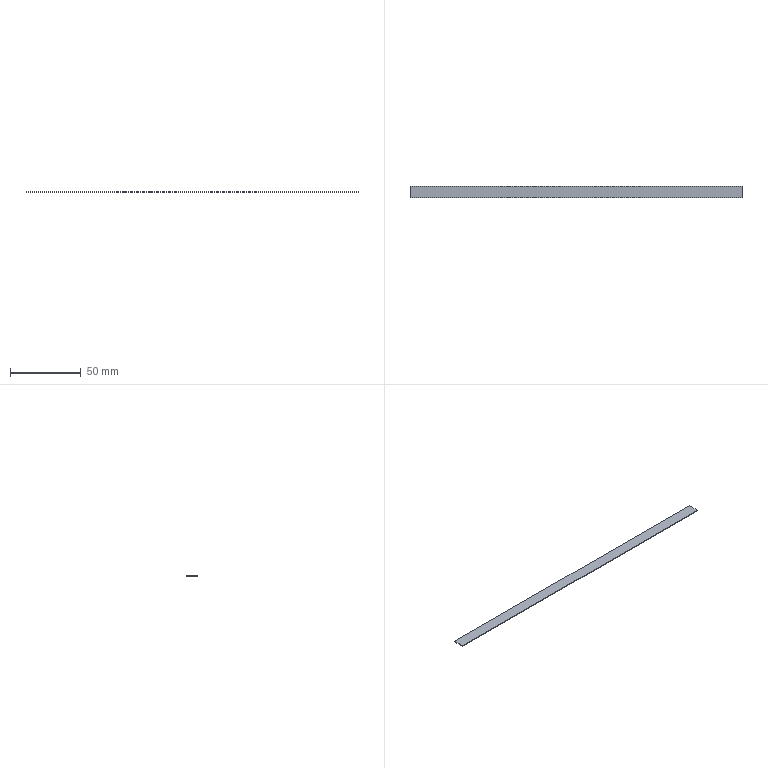Part | STEP file | 1 solid | 6 faces | box 235 x 8 x 0.5 mm | volume 940 mm3 | plane 6
STEP:
#1=CARTESIAN_POINT('',(0.,0.,0.));
#2=DIRECTION('',(0.,0.,1.));
#3=DIRECTION('',(1.,0.,0.));
#4=AXIS2_PLACEMENT_3D('',#1,#2,#3);
#5=CARTESIAN_POINT('',(117.5,-4.,0.));
#6=VERTEX_POINT('',#5);
#7=CARTESIAN_POINT('',(117.5,4.,0.));
#8=VERTEX_POINT('',#7);
#9=CARTESIAN_POINT('',(117.5,-4.,0.));
#10=DIRECTION('',(0.,1.,0.));
#11=VECTOR('',#10,1.);
#12=LINE('',#9,#11);
#13=CARTESIAN_POINT('',(0.,0.,0.));
#14=DIRECTION('',(0.,0.,-1.));
#15=DIRECTION('',(-1.,0.,0.));
#16=AXIS2_PLACEMENT_3D('',#13,#14,#15);
#17=PLANE('',#16);
#18=CARTESIAN_POINT('',(-117.5,-4.));
#19=DIRECTION('',(0.,1.));
#20=VECTOR('',#19,1.);
#21=LINE('',#18,#20);
#22=(GEOMETRIC_REPRESENTATION_CONTEXT(2)PARAMETRIC_REPRESENTATION_CONTEXT()REPRESENTATION_CONTEXT('',''));
#23=DEFINITIONAL_REPRESENTATION('',(#21),#22);
#24=PCURVE('',#17,#23);
#25=CARTESIAN_POINT('',(117.5,-4.,0.5));
#26=DIRECTION('',(-1.,0.,0.));
#27=DIRECTION('',(0.,0.,1.));
#28=AXIS2_PLACEMENT_3D('',#25,#26,#27);
#29=PLANE('',#28);
#30=CARTESIAN_POINT('',(-0.5,0.));
#31=DIRECTION('',(0.,1.));
#32=VECTOR('',#31,1.);
#33=LINE('',#30,#32);
#34=(GEOMETRIC_REPRESENTATION_CONTEXT(2)PARAMETRIC_REPRESENTATION_CONTEXT()REPRESENTATION_CONTEXT('',''));
#35=DEFINITIONAL_REPRESENTATION('',(#33),#34);
#36=PCURVE('',#29,#35);
#37=SURFACE_CURVE('',#12,(#24,#36),.PCURVE_S1.);
#38=EDGE_CURVE('',#6,#8,#37,.T.);
#39=ORIENTED_EDGE('',*,*,#38,.F.);
#40=CARTESIAN_POINT('',(-117.5,-4.,0.));
#41=VERTEX_POINT('',#40);
#42=CARTESIAN_POINT('',(-117.5,-4.,0.));
#43=DIRECTION('',(1.,0.,0.));
#44=VECTOR('',#43,1.);
#45=LINE('',#42,#44);
#46=CARTESIAN_POINT('',(117.5,-4.));
#47=DIRECTION('',(-1.,0.));
#48=VECTOR('',#47,1.);
#49=LINE('',#46,#48);
#50=(GEOMETRIC_REPRESENTATION_CONTEXT(2)PARAMETRIC_REPRESENTATION_CONTEXT()REPRESENTATION_CONTEXT('',''));
#51=DEFINITIONAL_REPRESENTATION('',(#49),#50);
#52=PCURVE('',#17,#51);
#53=CARTESIAN_POINT('',(-117.5,-4.,0.5));
#54=DIRECTION('',(0.,1.,0.));
#55=DIRECTION('',(0.,0.,1.));
#56=AXIS2_PLACEMENT_3D('',#53,#54,#55);
#57=PLANE('',#56);
#58=CARTESIAN_POINT('',(-0.5,0.));
#59=DIRECTION('',(0.,1.));
#60=VECTOR('',#59,1.);
#61=LINE('',#58,#60);
#62=(GEOMETRIC_REPRESENTATION_CONTEXT(2)PARAMETRIC_REPRESENTATION_CONTEXT()REPRESENTATION_CONTEXT('',''));
#63=DEFINITIONAL_REPRESENTATION('',(#61),#62);
#64=PCURVE('',#57,#63);
#65=SURFACE_CURVE('',#45,(#52,#64),.PCURVE_S1.);
#66=EDGE_CURVE('',#41,#6,#65,.T.);
#67=ORIENTED_EDGE('',*,*,#66,.F.);
#68=CARTESIAN_POINT('',(-117.5,4.,0.));
#69=VERTEX_POINT('',#68);
#70=CARTESIAN_POINT('',(-117.5,-4.,0.));
#71=DIRECTION('',(0.,-1.,0.));
#72=VECTOR('',#71,1.);
#73=LINE('',#70,#72);
#74=CARTESIAN_POINT('',(117.5,-4.));
#75=DIRECTION('',(0.,-1.));
#76=VECTOR('',#75,1.);
#77=LINE('',#74,#76);
#78=(GEOMETRIC_REPRESENTATION_CONTEXT(2)PARAMETRIC_REPRESENTATION_CONTEXT()REPRESENTATION_CONTEXT('',''));
#79=DEFINITIONAL_REPRESENTATION('',(#77),#78);
#80=PCURVE('',#17,#79);
#81=CARTESIAN_POINT('',(-117.5,-4.,0.5));
#82=DIRECTION('',(1.,0.,0.));
#83=DIRECTION('',(0.,0.,-1.));
#84=AXIS2_PLACEMENT_3D('',#81,#82,#83);
#85=PLANE('',#84);
#86=CARTESIAN_POINT('',(0.5,0.));
#87=DIRECTION('',(0.,-1.));
#88=VECTOR('',#87,1.);
#89=LINE('',#86,#88);
#90=(GEOMETRIC_REPRESENTATION_CONTEXT(2)PARAMETRIC_REPRESENTATION_CONTEXT()REPRESENTATION_CONTEXT('',''));
#91=DEFINITIONAL_REPRESENTATION('',(#89),#90);
#92=PCURVE('',#85,#91);
#93=SURFACE_CURVE('',#73,(#80,#92),.PCURVE_S1.);
#94=EDGE_CURVE('',#69,#41,#93,.T.);
#95=ORIENTED_EDGE('',*,*,#94,.F.);
#96=CARTESIAN_POINT('',(-117.5,4.,0.));
#97=DIRECTION('',(-1.,0.,0.));
#98=VECTOR('',#97,1.);
#99=LINE('',#96,#98);
#100=CARTESIAN_POINT('',(117.5,4.));
#101=DIRECTION('',(1.,0.));
#102=VECTOR('',#101,1.);
#103=LINE('',#100,#102);
#104=(GEOMETRIC_REPRESENTATION_CONTEXT(2)PARAMETRIC_REPRESENTATION_CONTEXT()REPRESENTATION_CONTEXT('',''));
#105=DEFINITIONAL_REPRESENTATION('',(#103),#104);
#106=PCURVE('',#17,#105);
#107=CARTESIAN_POINT('',(-117.5,4.,0.5));
#108=DIRECTION('',(0.,-1.,0.));
#109=DIRECTION('',(0.,0.,-1.));
#110=AXIS2_PLACEMENT_3D('',#107,#108,#109);
#111=PLANE('',#110);
#112=CARTESIAN_POINT('',(0.5,0.));
#113=DIRECTION('',(0.,-1.));
#114=VECTOR('',#113,1.);
#115=LINE('',#112,#114);
#116=(GEOMETRIC_REPRESENTATION_CONTEXT(2)PARAMETRIC_REPRESENTATION_CONTEXT()REPRESENTATION_CONTEXT('',''));
#117=DEFINITIONAL_REPRESENTATION('',(#115),#116);
#118=PCURVE('',#111,#117);
#119=SURFACE_CURVE('',#99,(#106,#118),.PCURVE_S1.);
#120=EDGE_CURVE('',#8,#69,#119,.T.);
#121=ORIENTED_EDGE('',*,*,#120,.F.);
#122=EDGE_LOOP('',(#39,#67,#95,#121));
#123=FACE_BOUND('',#122,.T.);
#124=ADVANCED_FACE('',(#123),#17,.T.);
#125=CARTESIAN_POINT('',(117.5,-4.,0.5));
#126=VERTEX_POINT('',#125);
#127=CARTESIAN_POINT('',(117.5,4.,0.5));
#128=VERTEX_POINT('',#127);
#129=CARTESIAN_POINT('',(117.5,-4.,0.5));
#130=DIRECTION('',(0.,1.,0.));
#131=VECTOR('',#130,1.);
#132=LINE('',#129,#131);
#133=CARTESIAN_POINT('',(0.,0.,0.5));
#134=DIRECTION('',(0.,0.,-1.));
#135=DIRECTION('',(-1.,0.,0.));
#136=AXIS2_PLACEMENT_3D('',#133,#134,#135);
#137=PLANE('',#136);
#138=CARTESIAN_POINT('',(-117.5,-4.));
#139=DIRECTION('',(0.,1.));
#140=VECTOR('',#139,1.);
#141=LINE('',#138,#140);
#142=(GEOMETRIC_REPRESENTATION_CONTEXT(2)PARAMETRIC_REPRESENTATION_CONTEXT()REPRESENTATION_CONTEXT('',''));
#143=DEFINITIONAL_REPRESENTATION('',(#141),#142);
#144=PCURVE('',#137,#143);
#145=CARTESIAN_POINT('',(0.,0.));
#146=DIRECTION('',(0.,1.));
#147=VECTOR('',#146,1.);
#148=LINE('',#145,#147);
#149=(GEOMETRIC_REPRESENTATION_CONTEXT(2)PARAMETRIC_REPRESENTATION_CONTEXT()REPRESENTATION_CONTEXT('',''));
#150=DEFINITIONAL_REPRESENTATION('',(#148),#149);
#151=PCURVE('',#29,#150);
#152=SURFACE_CURVE('',#132,(#144,#151),.PCURVE_S1.);
#153=EDGE_CURVE('',#126,#128,#152,.T.);
#154=ORIENTED_EDGE('',*,*,#153,.T.);
#155=CARTESIAN_POINT('',(-117.5,4.,0.5));
#156=VERTEX_POINT('',#155);
#157=CARTESIAN_POINT('',(-117.5,4.,0.5));
#158=DIRECTION('',(-1.,0.,0.));
#159=VECTOR('',#158,1.);
#160=LINE('',#157,#159);
#161=CARTESIAN_POINT('',(117.5,4.));
#162=DIRECTION('',(1.,0.));
#163=VECTOR('',#162,1.);
#164=LINE('',#161,#163);
#165=(GEOMETRIC_REPRESENTATION_CONTEXT(2)PARAMETRIC_REPRESENTATION_CONTEXT()REPRESENTATION_CONTEXT('',''));
#166=DEFINITIONAL_REPRESENTATION('',(#164),#165);
#167=PCURVE('',#137,#166);
#168=CARTESIAN_POINT('',(0.,0.));
#169=DIRECTION('',(0.,-1.));
#170=VECTOR('',#169,1.);
#171=LINE('',#168,#170);
#172=(GEOMETRIC_REPRESENTATION_CONTEXT(2)PARAMETRIC_REPRESENTATION_CONTEXT()REPRESENTATION_CONTEXT('',''));
#173=DEFINITIONAL_REPRESENTATION('',(#171),#172);
#174=PCURVE('',#111,#173);
#175=SURFACE_CURVE('',#160,(#167,#174),.PCURVE_S1.);
#176=EDGE_CURVE('',#128,#156,#175,.T.);
#177=ORIENTED_EDGE('',*,*,#176,.T.);
#178=CARTESIAN_POINT('',(-117.5,-4.,0.5));
#179=VERTEX_POINT('',#178);
#180=CARTESIAN_POINT('',(-117.5,-4.,0.5));
#181=DIRECTION('',(0.,-1.,0.));
#182=VECTOR('',#181,1.);
#183=LINE('',#180,#182);
#184=CARTESIAN_POINT('',(117.5,-4.));
#185=DIRECTION('',(0.,-1.));
#186=VECTOR('',#185,1.);
#187=LINE('',#184,#186);
#188=(GEOMETRIC_REPRESENTATION_CONTEXT(2)PARAMETRIC_REPRESENTATION_CONTEXT()REPRESENTATION_CONTEXT('',''));
#189=DEFINITIONAL_REPRESENTATION('',(#187),#188);
#190=PCURVE('',#137,#189);
#191=CARTESIAN_POINT('',(0.,0.));
#192=DIRECTION('',(0.,-1.));
#193=VECTOR('',#192,1.);
#194=LINE('',#191,#193);
#195=(GEOMETRIC_REPRESENTATION_CONTEXT(2)PARAMETRIC_REPRESENTATION_CONTEXT()REPRESENTATION_CONTEXT('',''));
#196=DEFINITIONAL_REPRESENTATION('',(#194),#195);
#197=PCURVE('',#85,#196);
#198=SURFACE_CURVE('',#183,(#190,#197),.PCURVE_S1.);
#199=EDGE_CURVE('',#156,#179,#198,.T.);
#200=ORIENTED_EDGE('',*,*,#199,.T.);
#201=CARTESIAN_POINT('',(-117.5,-4.,0.5));
#202=DIRECTION('',(1.,0.,0.));
#203=VECTOR('',#202,1.);
#204=LINE('',#201,#203);
#205=CARTESIAN_POINT('',(117.5,-4.));
#206=DIRECTION('',(-1.,0.));
#207=VECTOR('',#206,1.);
#208=LINE('',#205,#207);
#209=(GEOMETRIC_REPRESENTATION_CONTEXT(2)PARAMETRIC_REPRESENTATION_CONTEXT()REPRESENTATION_CONTEXT('',''));
#210=DEFINITIONAL_REPRESENTATION('',(#208),#209);
#211=PCURVE('',#137,#210);
#212=CARTESIAN_POINT('',(0.,0.));
#213=DIRECTION('',(0.,1.));
#214=VECTOR('',#213,1.);
#215=LINE('',#212,#214);
#216=(GEOMETRIC_REPRESENTATION_CONTEXT(2)PARAMETRIC_REPRESENTATION_CONTEXT()REPRESENTATION_CONTEXT('',''));
#217=DEFINITIONAL_REPRESENTATION('',(#215),#216);
#218=PCURVE('',#57,#217);
#219=SURFACE_CURVE('',#204,(#211,#218),.PCURVE_S1.);
#220=EDGE_CURVE('',#179,#126,#219,.T.);
#221=ORIENTED_EDGE('',*,*,#220,.T.);
#222=EDGE_LOOP('',(#154,#177,#200,#221));
#223=FACE_BOUND('',#222,.T.);
#224=ADVANCED_FACE('',(#223),#137,.F.);
#225=ORIENTED_EDGE('',*,*,#66,.T.);
#226=CARTESIAN_POINT('',(117.5,-4.,0.5));
#227=DIRECTION('',(0.,0.,-1.));
#228=VECTOR('',#227,1.);
#229=LINE('',#226,#228);
#230=CARTESIAN_POINT('',(0.,235.));
#231=DIRECTION('',(-1.,0.));
#232=VECTOR('',#231,1.);
#233=LINE('',#230,#232);
#234=(GEOMETRIC_REPRESENTATION_CONTEXT(2)PARAMETRIC_REPRESENTATION_CONTEXT()REPRESENTATION_CONTEXT('',''));
#235=DEFINITIONAL_REPRESENTATION('',(#233),#234);
#236=PCURVE('',#57,#235);
#237=CARTESIAN_POINT('',(0.,0.));
#238=DIRECTION('',(-1.,0.));
#239=VECTOR('',#238,1.);
#240=LINE('',#237,#239);
#241=(GEOMETRIC_REPRESENTATION_CONTEXT(2)PARAMETRIC_REPRESENTATION_CONTEXT()REPRESENTATION_CONTEXT('',''));
#242=DEFINITIONAL_REPRESENTATION('',(#240),#241);
#243=PCURVE('',#29,#242);
#244=SURFACE_CURVE('',#229,(#236,#243),.PCURVE_S1.);
#245=EDGE_CURVE('',#126,#6,#244,.T.);
#246=ORIENTED_EDGE('',*,*,#245,.F.);
#247=ORIENTED_EDGE('',*,*,#220,.F.);
#248=CARTESIAN_POINT('',(-117.5,-4.,0.5));
#249=DIRECTION('',(0.,0.,-1.));
#250=VECTOR('',#249,1.);
#251=LINE('',#248,#250);
#252=CARTESIAN_POINT('',(0.,0.));
#253=DIRECTION('',(-1.,0.));
#254=VECTOR('',#253,1.);
#255=LINE('',#252,#254);
#256=(GEOMETRIC_REPRESENTATION_CONTEXT(2)PARAMETRIC_REPRESENTATION_CONTEXT()REPRESENTATION_CONTEXT('',''));
#257=DEFINITIONAL_REPRESENTATION('',(#255),#256);
#258=PCURVE('',#57,#257);
#259=CARTESIAN_POINT('',(0.,0.));
#260=DIRECTION('',(1.,0.));
#261=VECTOR('',#260,1.);
#262=LINE('',#259,#261);
#263=(GEOMETRIC_REPRESENTATION_CONTEXT(2)PARAMETRIC_REPRESENTATION_CONTEXT()REPRESENTATION_CONTEXT('',''));
#264=DEFINITIONAL_REPRESENTATION('',(#262),#263);
#265=PCURVE('',#85,#264);
#266=SURFACE_CURVE('',#251,(#258,#265),.PCURVE_S1.);
#267=EDGE_CURVE('',#179,#41,#266,.T.);
#268=ORIENTED_EDGE('',*,*,#267,.T.);
#269=EDGE_LOOP('',(#225,#246,#247,#268));
#270=FACE_BOUND('',#269,.T.);
#271=ADVANCED_FACE('',(#270),#57,.F.);
#272=ORIENTED_EDGE('',*,*,#94,.T.);
#273=ORIENTED_EDGE('',*,*,#267,.F.);
#274=ORIENTED_EDGE('',*,*,#199,.F.);
#275=CARTESIAN_POINT('',(-117.5,4.,0.5));
#276=DIRECTION('',(0.,0.,-1.));
#277=VECTOR('',#276,1.);
#278=LINE('',#275,#277);
#279=CARTESIAN_POINT('',(0.,8.));
#280=DIRECTION('',(1.,0.));
#281=VECTOR('',#280,1.);
#282=LINE('',#279,#281);
#283=(GEOMETRIC_REPRESENTATION_CONTEXT(2)PARAMETRIC_REPRESENTATION_CONTEXT()REPRESENTATION_CONTEXT('',''));
#284=DEFINITIONAL_REPRESENTATION('',(#282),#283);
#285=PCURVE('',#85,#284);
#286=CARTESIAN_POINT('',(0.,0.));
#287=DIRECTION('',(1.,0.));
#288=VECTOR('',#287,1.);
#289=LINE('',#286,#288);
#290=(GEOMETRIC_REPRESENTATION_CONTEXT(2)PARAMETRIC_REPRESENTATION_CONTEXT()REPRESENTATION_CONTEXT('',''));
#291=DEFINITIONAL_REPRESENTATION('',(#289),#290);
#292=PCURVE('',#111,#291);
#293=SURFACE_CURVE('',#278,(#285,#292),.PCURVE_S1.);
#294=EDGE_CURVE('',#156,#69,#293,.T.);
#295=ORIENTED_EDGE('',*,*,#294,.T.);
#296=EDGE_LOOP('',(#272,#273,#274,#295));
#297=FACE_BOUND('',#296,.T.);
#298=ADVANCED_FACE('',(#297),#85,.F.);
#299=ORIENTED_EDGE('',*,*,#120,.T.);
#300=ORIENTED_EDGE('',*,*,#294,.F.);
#301=ORIENTED_EDGE('',*,*,#176,.F.);
#302=CARTESIAN_POINT('',(117.5,4.,0.5));
#303=DIRECTION('',(0.,0.,-1.));
#304=VECTOR('',#303,1.);
#305=LINE('',#302,#304);
#306=CARTESIAN_POINT('',(0.,235.));
#307=DIRECTION('',(1.,0.));
#308=VECTOR('',#307,1.);
#309=LINE('',#306,#308);
#310=(GEOMETRIC_REPRESENTATION_CONTEXT(2)PARAMETRIC_REPRESENTATION_CONTEXT()REPRESENTATION_CONTEXT('',''));
#311=DEFINITIONAL_REPRESENTATION('',(#309),#310);
#312=PCURVE('',#111,#311);
#313=CARTESIAN_POINT('',(0.,8.));
#314=DIRECTION('',(-1.,0.));
#315=VECTOR('',#314,1.);
#316=LINE('',#313,#315);
#317=(GEOMETRIC_REPRESENTATION_CONTEXT(2)PARAMETRIC_REPRESENTATION_CONTEXT()REPRESENTATION_CONTEXT('',''));
#318=DEFINITIONAL_REPRESENTATION('',(#316),#317);
#319=PCURVE('',#29,#318);
#320=SURFACE_CURVE('',#305,(#312,#319),.PCURVE_S1.);
#321=EDGE_CURVE('',#128,#8,#320,.T.);
#322=ORIENTED_EDGE('',*,*,#321,.T.);
#323=EDGE_LOOP('',(#299,#300,#301,#322));
#324=FACE_BOUND('',#323,.T.);
#325=ADVANCED_FACE('',(#324),#111,.F.);
#326=ORIENTED_EDGE('',*,*,#38,.T.);
#327=ORIENTED_EDGE('',*,*,#321,.F.);
#328=ORIENTED_EDGE('',*,*,#153,.F.);
#329=ORIENTED_EDGE('',*,*,#245,.T.);
#330=EDGE_LOOP('',(#326,#327,#328,#329));
#331=FACE_BOUND('',#330,.T.);
#332=ADVANCED_FACE('',(#331),#29,.F.);
#333=CLOSED_SHELL('',(#124,#224,#271,#298,#325,#332));
#334=MANIFOLD_SOLID_BREP('',#333);
#335=(LENGTH_UNIT()NAMED_UNIT(*)SI_UNIT(.MILLI.,.METRE.));
#336=UNCERTAINTY_MEASURE_WITH_UNIT(LENGTH_MEASURE(0.0000001),#335,'','');
#337=(NAMED_UNIT(*)PLANE_ANGLE_UNIT()SI_UNIT($,.RADIAN.));
#338=(NAMED_UNIT(*)SI_UNIT($,.STERADIAN.)SOLID_ANGLE_UNIT());
#339=(GEOMETRIC_REPRESENTATION_CONTEXT(3)GLOBAL_UNCERTAINTY_ASSIGNED_CONTEXT((#336))GLOBAL_UNIT_ASSIGNED_CONTEXT((#335,#337,#338))REPRESENTATION_CONTEXT('',''));
#340=ADVANCED_BREP_SHAPE_REPRESENTATION('',(#4,#334),#339);